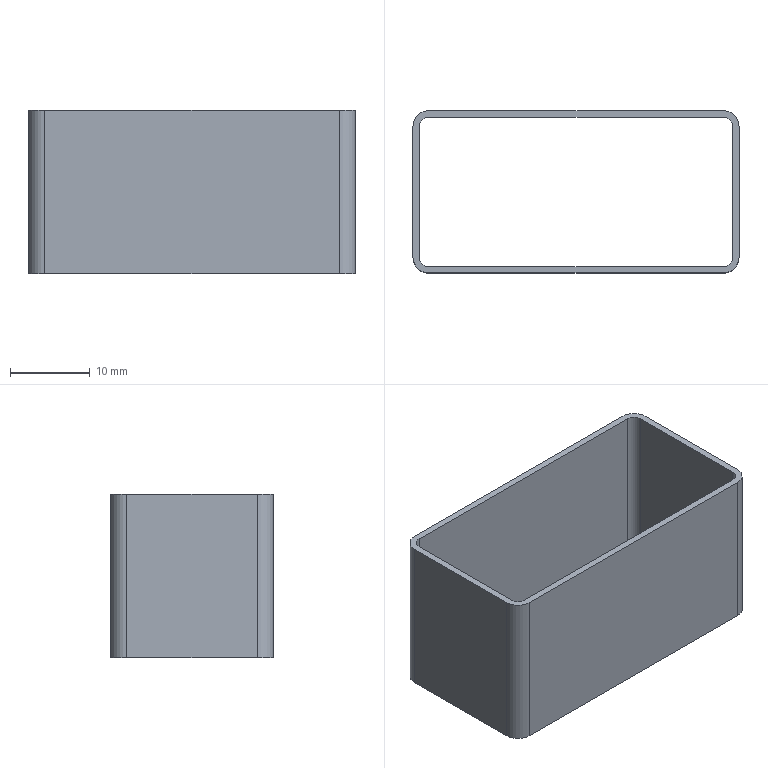Part | STEP file | Zapas-OpenRC Truggy HSPr v2. v55-3 | 1 solid | 18 faces | box 41 x 20.4 x 20.5 mm | volume 1916 mm3 | plane 10 | cylinder 8 | commonest cylinder face diameters 2.4 x4 4 x4
STEP:
#1=CARTESIAN_POINT('',(0.,0.,0.));
#2=DIRECTION('',(0.,0.,1.));
#3=DIRECTION('',(1.,0.,0.));
#4=AXIS2_PLACEMENT_3D('',#1,#2,#3);
#5=CARTESIAN_POINT('',(-21.509,42.508,-107.898));
#6=VERTEX_POINT('',#5);
#7=CARTESIAN_POINT('',(-21.509,42.508,-128.398));
#8=VERTEX_POINT('',#7);
#9=CARTESIAN_POINT('',(-21.509,42.508,-107.898));
#10=DIRECTION('',(0.,0.,-1.));
#11=VECTOR('',#10,1.);
#12=LINE('',#9,#11);
#13=CARTESIAN_POINT('',(-3.009,42.508,-118.148));
#14=DIRECTION('',(0.00000009,-1.,0.));
#15=DIRECTION('',(1.,0.00000009,0.));
#16=AXIS2_PLACEMENT_3D('',#13,#14,#15);
#17=PLANE('',#16);
#18=CARTESIAN_POINT('',(-18.5,10.25));
#19=DIRECTION('',(0.,-1.));
#20=VECTOR('',#19,1.);
#21=LINE('',#18,#20);
#22=(GEOMETRIC_REPRESENTATION_CONTEXT(2)PARAMETRIC_REPRESENTATION_CONTEXT()REPRESENTATION_CONTEXT('',''));
#23=DEFINITIONAL_REPRESENTATION('',(#21),#22);
#24=PCURVE('',#17,#23);
#25=CARTESIAN_POINT('',(-21.509,40.508,-107.898));
#26=DIRECTION('',(0.,0.,-1.));
#27=DIRECTION('',(1.,-0.00000091,0.));
#28=AXIS2_PLACEMENT_3D('',#25,#26,#27);
#29=CYLINDRICAL_SURFACE('',#28,2.);
#30=CARTESIAN_POINT('',(4.712,0.));
#31=DIRECTION('',(0.,1.));
#32=VECTOR('',#31,1.);
#33=LINE('',#30,#32);
#34=(GEOMETRIC_REPRESENTATION_CONTEXT(2)PARAMETRIC_REPRESENTATION_CONTEXT()REPRESENTATION_CONTEXT('',''));
#35=DEFINITIONAL_REPRESENTATION('',(#33),#34);
#36=PCURVE('',#29,#35);
#37=SURFACE_CURVE('',#12,(#24,#36),.PCURVE_S1.);
#38=EDGE_CURVE('',#6,#8,#37,.T.);
#39=ORIENTED_EDGE('',*,*,#38,.F.);
#40=CARTESIAN_POINT('',(15.491,42.508,-107.898));
#41=VERTEX_POINT('',#40);
#42=CARTESIAN_POINT('',(15.491,42.508,-107.898));
#43=DIRECTION('',(-1.,-0.00000009,0.));
#44=VECTOR('',#43,1.);
#45=LINE('',#42,#44);
#46=CARTESIAN_POINT('',(18.5,10.25));
#47=DIRECTION('',(-1.,0.));
#48=VECTOR('',#47,1.);
#49=LINE('',#46,#48);
#50=(GEOMETRIC_REPRESENTATION_CONTEXT(2)PARAMETRIC_REPRESENTATION_CONTEXT()REPRESENTATION_CONTEXT('',''));
#51=DEFINITIONAL_REPRESENTATION('',(#49),#50);
#52=PCURVE('',#17,#51);
#53=CARTESIAN_POINT('',(-3.009,32.308,-107.898));
#54=DIRECTION('',(0.,0.,1.));
#55=DIRECTION('',(-1.,0.00000091,0.));
#56=AXIS2_PLACEMENT_3D('',#53,#54,#55);
#57=PLANE('',#56);
#58=CARTESIAN_POINT('',(-18.5,-10.2));
#59=DIRECTION('',(1.,0.000001));
#60=VECTOR('',#59,1.);
#61=LINE('',#58,#60);
#62=(GEOMETRIC_REPRESENTATION_CONTEXT(2)PARAMETRIC_REPRESENTATION_CONTEXT()REPRESENTATION_CONTEXT('',''));
#63=DEFINITIONAL_REPRESENTATION('',(#61),#62);
#64=PCURVE('',#57,#63);
#65=SURFACE_CURVE('',#45,(#52,#64),.PCURVE_S1.);
#66=EDGE_CURVE('',#41,#6,#65,.T.);
#67=ORIENTED_EDGE('',*,*,#66,.F.);
#68=CARTESIAN_POINT('',(15.491,42.508,-128.398));
#69=VERTEX_POINT('',#68);
#70=CARTESIAN_POINT('',(15.491,42.508,-128.398));
#71=DIRECTION('',(0.,0.,1.));
#72=VECTOR('',#71,1.);
#73=LINE('',#70,#72);
#74=CARTESIAN_POINT('',(18.5,-10.25));
#75=DIRECTION('',(0.,1.));
#76=VECTOR('',#75,1.);
#77=LINE('',#74,#76);
#78=(GEOMETRIC_REPRESENTATION_CONTEXT(2)PARAMETRIC_REPRESENTATION_CONTEXT()REPRESENTATION_CONTEXT('',''));
#79=DEFINITIONAL_REPRESENTATION('',(#77),#78);
#80=PCURVE('',#17,#79);
#81=CARTESIAN_POINT('',(15.491,40.508,-107.898));
#82=DIRECTION('',(0.,0.,-1.));
#83=DIRECTION('',(1.,-0.00000091,0.));
#84=AXIS2_PLACEMENT_3D('',#81,#82,#83);
#85=CYLINDRICAL_SURFACE('',#84,2.);
#86=CARTESIAN_POINT('',(4.712,20.5));
#87=DIRECTION('',(0.,-1.));
#88=VECTOR('',#87,1.);
#89=LINE('',#86,#88);
#90=(GEOMETRIC_REPRESENTATION_CONTEXT(2)PARAMETRIC_REPRESENTATION_CONTEXT()REPRESENTATION_CONTEXT('',''));
#91=DEFINITIONAL_REPRESENTATION('',(#89),#90);
#92=PCURVE('',#85,#91);
#93=SURFACE_CURVE('',#73,(#80,#92),.PCURVE_S1.);
#94=EDGE_CURVE('',#69,#41,#93,.T.);
#95=ORIENTED_EDGE('',*,*,#94,.F.);
#96=CARTESIAN_POINT('',(-21.509,42.508,-128.398));
#97=DIRECTION('',(1.,0.00000009,0.));
#98=VECTOR('',#97,1.);
#99=LINE('',#96,#98);
#100=CARTESIAN_POINT('',(-18.5,-10.25));
#101=DIRECTION('',(1.,0.));
#102=VECTOR('',#101,1.);
#103=LINE('',#100,#102);
#104=(GEOMETRIC_REPRESENTATION_CONTEXT(2)PARAMETRIC_REPRESENTATION_CONTEXT()REPRESENTATION_CONTEXT('',''));
#105=DEFINITIONAL_REPRESENTATION('',(#103),#104);
#106=PCURVE('',#17,#105);
#107=CARTESIAN_POINT('',(-3.009,32.308,-128.398));
#108=DIRECTION('',(0.,0.,1.));
#109=DIRECTION('',(-1.,0.00000091,0.));
#110=AXIS2_PLACEMENT_3D('',#107,#108,#109);
#111=PLANE('',#110);
#112=CARTESIAN_POINT('',(18.5,-10.2));
#113=DIRECTION('',(-1.,-0.000001));
#114=VECTOR('',#113,1.);
#115=LINE('',#112,#114);
#116=(GEOMETRIC_REPRESENTATION_CONTEXT(2)PARAMETRIC_REPRESENTATION_CONTEXT()REPRESENTATION_CONTEXT('',''));
#117=DEFINITIONAL_REPRESENTATION('',(#115),#116);
#118=PCURVE('',#111,#117);
#119=SURFACE_CURVE('',#99,(#106,#118),.PCURVE_S1.);
#120=EDGE_CURVE('',#8,#69,#119,.T.);
#121=ORIENTED_EDGE('',*,*,#120,.F.);
#122=EDGE_LOOP('',(#39,#67,#95,#121));
#123=FACE_BOUND('',#122,.T.);
#124=ADVANCED_FACE('',(#123),#17,.F.);
#125=CARTESIAN_POINT('',(-22.709,40.508,-128.398));
#126=VERTEX_POINT('',#125);
#127=CARTESIAN_POINT('',(-21.509,41.708,-128.398));
#128=VERTEX_POINT('',#127);
#129=CARTESIAN_POINT('',(-21.509,40.508,-128.398));
#130=DIRECTION('',(0.,0.,-1.));
#131=DIRECTION('',(-1.,0.00000091,0.));
#132=AXIS2_PLACEMENT_3D('',#129,#130,#131);
#133=CIRCLE('',#132,1.2);
#134=CARTESIAN_POINT('',(19.7,-8.2));
#135=CARTESIAN_POINT('',(19.7,-10.278));
#136=CARTESIAN_POINT('',(17.9,-9.239));
#137=CARTESIAN_POINT('',(16.1,-8.2));
#138=CARTESIAN_POINT('',(17.9,-7.161));
#139=CARTESIAN_POINT('',(19.7,-6.122));
#140=CARTESIAN_POINT('',(19.7,-8.2));
#141=(BOUNDED_CURVE()B_SPLINE_CURVE(2,(#134,#135,#136,#137,#138,#139,#140),.UNSPECIFIED.,.T.,.F.)B_SPLINE_CURVE_WITH_KNOTS((1,2,2,2,2,1),(-2.094,0.,2.094,4.189,6.283,8.378),.UNSPECIFIED.)CURVE()GEOMETRIC_REPRESENTATION_ITEM()RATIONAL_B_SPLINE_CURVE((1.,0.5,1.,0.5,1.,0.5,1.))REPRESENTATION_ITEM(''));
#142=(GEOMETRIC_REPRESENTATION_CONTEXT(2)PARAMETRIC_REPRESENTATION_CONTEXT()REPRESENTATION_CONTEXT('',''));
#143=DEFINITIONAL_REPRESENTATION('',(#141),#142);
#144=PCURVE('',#111,#143);
#145=CARTESIAN_POINT('',(-21.509,40.508,-128.398));
#146=DIRECTION('',(0.,0.,1.));
#147=DIRECTION('',(-1.,0.00000091,0.));
#148=AXIS2_PLACEMENT_3D('',#145,#146,#147);
#149=CYLINDRICAL_SURFACE('',#148,1.2);
#150=CARTESIAN_POINT('',(12.566,0.));
#151=DIRECTION('',(-1.,0.));
#152=VECTOR('',#151,1.);
#153=LINE('',#150,#152);
#154=(GEOMETRIC_REPRESENTATION_CONTEXT(2)PARAMETRIC_REPRESENTATION_CONTEXT()REPRESENTATION_CONTEXT('',''));
#155=DEFINITIONAL_REPRESENTATION('',(#153),#154);
#156=PCURVE('',#149,#155);
#157=SURFACE_CURVE('',#133,(#144,#156),.PCURVE_S1.);
#158=EDGE_CURVE('',#126,#128,#157,.T.);
#159=ORIENTED_EDGE('',*,*,#158,.F.);
#160=CARTESIAN_POINT('',(-22.709,24.108,-128.398));
#161=VERTEX_POINT('',#160);
#162=CARTESIAN_POINT('',(-22.709,24.108,-128.398));
#163=DIRECTION('',(-0.00000009,1.,0.));
#164=VECTOR('',#163,1.);
#165=LINE('',#162,#164);
#166=CARTESIAN_POINT('',(19.7,8.2));
#167=DIRECTION('',(0.000001,-1.));
#168=VECTOR('',#167,1.);
#169=LINE('',#166,#168);
#170=(GEOMETRIC_REPRESENTATION_CONTEXT(2)PARAMETRIC_REPRESENTATION_CONTEXT()REPRESENTATION_CONTEXT('',''));
#171=DEFINITIONAL_REPRESENTATION('',(#169),#170);
#172=PCURVE('',#111,#171);
#173=CARTESIAN_POINT('',(-22.709,32.308,-118.148));
#174=DIRECTION('',(-1.,-0.00000009,0.));
#175=DIRECTION('',(0.00000009,-1.,0.));
#176=AXIS2_PLACEMENT_3D('',#173,#174,#175);
#177=PLANE('',#176);
#178=CARTESIAN_POINT('',(8.2,-10.25));
#179=DIRECTION('',(-1.,0.));
#180=VECTOR('',#179,1.);
#181=LINE('',#178,#180);
#182=(GEOMETRIC_REPRESENTATION_CONTEXT(2)PARAMETRIC_REPRESENTATION_CONTEXT()REPRESENTATION_CONTEXT('',''));
#183=DEFINITIONAL_REPRESENTATION('',(#181),#182);
#184=PCURVE('',#177,#183);
#185=SURFACE_CURVE('',#165,(#172,#184),.PCURVE_S1.);
#186=EDGE_CURVE('',#161,#126,#185,.T.);
#187=ORIENTED_EDGE('',*,*,#186,.F.);
#188=CARTESIAN_POINT('',(-21.509,22.908,-128.398));
#189=VERTEX_POINT('',#188);
#190=CARTESIAN_POINT('',(-21.509,24.108,-128.398));
#191=DIRECTION('',(0.,0.,-1.));
#192=DIRECTION('',(-1.,0.00000091,0.));
#193=AXIS2_PLACEMENT_3D('',#190,#191,#192);
#194=CIRCLE('',#193,1.2);
#195=CARTESIAN_POINT('',(19.7,8.2));
#196=CARTESIAN_POINT('',(19.7,6.122));
#197=CARTESIAN_POINT('',(17.9,7.161));
#198=CARTESIAN_POINT('',(16.1,8.2));
#199=CARTESIAN_POINT('',(17.9,9.239));
#200=CARTESIAN_POINT('',(19.7,10.278));
#201=CARTESIAN_POINT('',(19.7,8.2));
#202=(BOUNDED_CURVE()B_SPLINE_CURVE(2,(#195,#196,#197,#198,#199,#200,#201),.UNSPECIFIED.,.T.,.F.)B_SPLINE_CURVE_WITH_KNOTS((1,2,2,2,2,1),(-2.094,0.,2.094,4.189,6.283,8.378),.UNSPECIFIED.)CURVE()GEOMETRIC_REPRESENTATION_ITEM()RATIONAL_B_SPLINE_CURVE((1.,0.5,1.,0.5,1.,0.5,1.))REPRESENTATION_ITEM(''));
#203=(GEOMETRIC_REPRESENTATION_CONTEXT(2)PARAMETRIC_REPRESENTATION_CONTEXT()REPRESENTATION_CONTEXT('',''));
#204=DEFINITIONAL_REPRESENTATION('',(#202),#203);
#205=PCURVE('',#111,#204);
#206=CARTESIAN_POINT('',(-21.509,24.108,-128.398));
#207=DIRECTION('',(0.,0.,1.));
#208=DIRECTION('',(-1.,0.00000091,0.));
#209=AXIS2_PLACEMENT_3D('',#206,#207,#208);
#210=CYLINDRICAL_SURFACE('',#209,1.2);
#211=CARTESIAN_POINT('',(6.283,0.));
#212=DIRECTION('',(-1.,0.));
#213=VECTOR('',#212,1.);
#214=LINE('',#211,#213);
#215=(GEOMETRIC_REPRESENTATION_CONTEXT(2)PARAMETRIC_REPRESENTATION_CONTEXT()REPRESENTATION_CONTEXT('',''));
#216=DEFINITIONAL_REPRESENTATION('',(#214),#215);
#217=PCURVE('',#210,#216);
#218=SURFACE_CURVE('',#194,(#205,#217),.PCURVE_S1.);
#219=EDGE_CURVE('',#189,#161,#218,.T.);
#220=ORIENTED_EDGE('',*,*,#219,.F.);
#221=CARTESIAN_POINT('',(15.491,22.908,-128.398));
#222=VERTEX_POINT('',#221);
#223=CARTESIAN_POINT('',(15.491,22.908,-128.398));
#224=DIRECTION('',(-1.,-0.00000009,0.));
#225=VECTOR('',#224,1.);
#226=LINE('',#223,#225);
#227=CARTESIAN_POINT('',(-18.5,9.4));
#228=DIRECTION('',(1.,0.000001));
#229=VECTOR('',#228,1.);
#230=LINE('',#227,#229);
#231=(GEOMETRIC_REPRESENTATION_CONTEXT(2)PARAMETRIC_REPRESENTATION_CONTEXT()REPRESENTATION_CONTEXT('',''));
#232=DEFINITIONAL_REPRESENTATION('',(#230),#231);
#233=PCURVE('',#111,#232);
#234=CARTESIAN_POINT('',(-3.009,22.908,-118.148));
#235=DIRECTION('',(0.00000009,-1.,0.));
#236=DIRECTION('',(1.,0.00000009,0.));
#237=AXIS2_PLACEMENT_3D('',#234,#235,#236);
#238=PLANE('',#237);
#239=CARTESIAN_POINT('',(18.5,-10.25));
#240=DIRECTION('',(-1.,0.));
#241=VECTOR('',#240,1.);
#242=LINE('',#239,#241);
#243=(GEOMETRIC_REPRESENTATION_CONTEXT(2)PARAMETRIC_REPRESENTATION_CONTEXT()REPRESENTATION_CONTEXT('',''));
#244=DEFINITIONAL_REPRESENTATION('',(#242),#243);
#245=PCURVE('',#238,#244);
#246=SURFACE_CURVE('',#226,(#233,#245),.PCURVE_S1.);
#247=EDGE_CURVE('',#222,#189,#246,.T.);
#248=ORIENTED_EDGE('',*,*,#247,.F.);
#249=CARTESIAN_POINT('',(16.691,24.108,-128.398));
#250=VERTEX_POINT('',#249);
#251=CARTESIAN_POINT('',(15.491,24.108,-128.398));
#252=DIRECTION('',(0.,0.,-1.));
#253=DIRECTION('',(-1.,0.00000091,0.));
#254=AXIS2_PLACEMENT_3D('',#251,#252,#253);
#255=CIRCLE('',#254,1.2);
#256=CARTESIAN_POINT('',(-17.3,8.2));
#257=CARTESIAN_POINT('',(-17.3,6.122));
#258=CARTESIAN_POINT('',(-19.1,7.161));
#259=CARTESIAN_POINT('',(-20.9,8.2));
#260=CARTESIAN_POINT('',(-19.1,9.239));
#261=CARTESIAN_POINT('',(-17.3,10.278));
#262=CARTESIAN_POINT('',(-17.3,8.2));
#263=(BOUNDED_CURVE()B_SPLINE_CURVE(2,(#256,#257,#258,#259,#260,#261,#262),.UNSPECIFIED.,.T.,.F.)B_SPLINE_CURVE_WITH_KNOTS((1,2,2,2,2,1),(-2.094,0.,2.094,4.189,6.283,8.378),.UNSPECIFIED.)CURVE()GEOMETRIC_REPRESENTATION_ITEM()RATIONAL_B_SPLINE_CURVE((1.,0.5,1.,0.5,1.,0.5,1.))REPRESENTATION_ITEM(''));
#264=(GEOMETRIC_REPRESENTATION_CONTEXT(2)PARAMETRIC_REPRESENTATION_CONTEXT()REPRESENTATION_CONTEXT('',''));
#265=DEFINITIONAL_REPRESENTATION('',(#263),#264);
#266=PCURVE('',#111,#265);
#267=CARTESIAN_POINT('',(15.491,24.108,-128.398));
#268=DIRECTION('',(0.,0.,1.));
#269=DIRECTION('',(-1.,0.00000091,0.));
#270=AXIS2_PLACEMENT_3D('',#267,#268,#269);
#271=CYLINDRICAL_SURFACE('',#270,1.2);
#272=CARTESIAN_POINT('',(6.283,0.));
#273=DIRECTION('',(-1.,0.));
#274=VECTOR('',#273,1.);
#275=LINE('',#272,#274);
#276=(GEOMETRIC_REPRESENTATION_CONTEXT(2)PARAMETRIC_REPRESENTATION_CONTEXT()REPRESENTATION_CONTEXT('',''));
#277=DEFINITIONAL_REPRESENTATION('',(#275),#276);
#278=PCURVE('',#271,#277);
#279=SURFACE_CURVE('',#255,(#266,#278),.PCURVE_S1.);
#280=EDGE_CURVE('',#250,#222,#279,.T.);
#281=ORIENTED_EDGE('',*,*,#280,.F.);
#282=CARTESIAN_POINT('',(16.691,40.508,-128.398));
#283=VERTEX_POINT('',#282);
#284=CARTESIAN_POINT('',(16.691,40.508,-128.398));
#285=DIRECTION('',(0.00000009,-1.,0.));
#286=VECTOR('',#285,1.);
#287=LINE('',#284,#286);
#288=CARTESIAN_POINT('',(-19.7,-8.2));
#289=DIRECTION('',(-0.000001,1.));
#290=VECTOR('',#289,1.);
#291=LINE('',#288,#290);
#292=(GEOMETRIC_REPRESENTATION_CONTEXT(2)PARAMETRIC_REPRESENTATION_CONTEXT()REPRESENTATION_CONTEXT('',''));
#293=DEFINITIONAL_REPRESENTATION('',(#291),#292);
#294=PCURVE('',#111,#293);
#295=CARTESIAN_POINT('',(16.691,32.308,-118.148));
#296=DIRECTION('',(1.,0.00000009,0.));
#297=DIRECTION('',(-0.00000009,1.,0.));
#298=AXIS2_PLACEMENT_3D('',#295,#296,#297);
#299=PLANE('',#298);
#300=CARTESIAN_POINT('',(8.2,-10.25));
#301=DIRECTION('',(-1.,0.));
#302=VECTOR('',#301,1.);
#303=LINE('',#300,#302);
#304=(GEOMETRIC_REPRESENTATION_CONTEXT(2)PARAMETRIC_REPRESENTATION_CONTEXT()REPRESENTATION_CONTEXT('',''));
#305=DEFINITIONAL_REPRESENTATION('',(#303),#304);
#306=PCURVE('',#299,#305);
#307=SURFACE_CURVE('',#287,(#294,#306),.PCURVE_S1.);
#308=EDGE_CURVE('',#283,#250,#307,.T.);
#309=ORIENTED_EDGE('',*,*,#308,.F.);
#310=CARTESIAN_POINT('',(15.491,41.708,-128.398));
#311=VERTEX_POINT('',#310);
#312=CARTESIAN_POINT('',(15.491,40.508,-128.398));
#313=DIRECTION('',(0.,0.,-1.));
#314=DIRECTION('',(-1.,0.00000091,0.));
#315=AXIS2_PLACEMENT_3D('',#312,#313,#314);
#316=CIRCLE('',#315,1.2);
#317=CARTESIAN_POINT('',(-17.3,-8.2));
#318=CARTESIAN_POINT('',(-17.3,-10.278));
#319=CARTESIAN_POINT('',(-19.1,-9.239));
#320=CARTESIAN_POINT('',(-20.9,-8.2));
#321=CARTESIAN_POINT('',(-19.1,-7.161));
#322=CARTESIAN_POINT('',(-17.3,-6.122));
#323=CARTESIAN_POINT('',(-17.3,-8.2));
#324=(BOUNDED_CURVE()B_SPLINE_CURVE(2,(#317,#318,#319,#320,#321,#322,#323),.UNSPECIFIED.,.T.,.F.)B_SPLINE_CURVE_WITH_KNOTS((1,2,2,2,2,1),(-2.094,0.,2.094,4.189,6.283,8.378),.UNSPECIFIED.)CURVE()GEOMETRIC_REPRESENTATION_ITEM()RATIONAL_B_SPLINE_CURVE((1.,0.5,1.,0.5,1.,0.5,1.))REPRESENTATION_ITEM(''));
#325=(GEOMETRIC_REPRESENTATION_CONTEXT(2)PARAMETRIC_REPRESENTATION_CONTEXT()REPRESENTATION_CONTEXT('',''));
#326=DEFINITIONAL_REPRESENTATION('',(#324),#325);
#327=PCURVE('',#111,#326);
#328=CARTESIAN_POINT('',(15.491,40.508,-128.398));
#329=DIRECTION('',(0.,0.,1.));
#330=DIRECTION('',(-1.,0.00000091,0.));
#331=AXIS2_PLACEMENT_3D('',#328,#329,#330);
#332=CYLINDRICAL_SURFACE('',#331,1.2);
#333=CARTESIAN_POINT('',(6.283,0.));
#334=DIRECTION('',(-1.,0.));
#335=VECTOR('',#334,1.);
#336=LINE('',#333,#335);
#337=(GEOMETRIC_REPRESENTATION_CONTEXT(2)PARAMETRIC_REPRESENTATION_CONTEXT()REPRESENTATION_CONTEXT('',''));
#338=DEFINITIONAL_REPRESENTATION('',(#336),#337);
#339=PCURVE('',#332,#338);
#340=SURFACE_CURVE('',#316,(#327,#339),.PCURVE_S1.);
#341=EDGE_CURVE('',#311,#283,#340,.T.);
#342=ORIENTED_EDGE('',*,*,#341,.F.);
#343=CARTESIAN_POINT('',(-21.509,41.708,-128.398));
#344=DIRECTION('',(1.,0.00000009,0.));
#345=VECTOR('',#344,1.);
#346=LINE('',#343,#345);
#347=CARTESIAN_POINT('',(18.5,-9.4));
#348=DIRECTION('',(-1.,-0.000001));
#349=VECTOR('',#348,1.);
#350=LINE('',#347,#349);
#351=(GEOMETRIC_REPRESENTATION_CONTEXT(2)PARAMETRIC_REPRESENTATION_CONTEXT()REPRESENTATION_CONTEXT('',''));
#352=DEFINITIONAL_REPRESENTATION('',(#350),#351);
#353=PCURVE('',#111,#352);
#354=CARTESIAN_POINT('',(-3.009,41.708,-118.148));
#355=DIRECTION('',(-0.00000009,1.,0.));
#356=DIRECTION('',(-1.,-0.00000009,0.));
#357=AXIS2_PLACEMENT_3D('',#354,#355,#356);
#358=PLANE('',#357);
#359=CARTESIAN_POINT('',(18.5,-10.25));
#360=DIRECTION('',(-1.,0.));
#361=VECTOR('',#360,1.);
#362=LINE('',#359,#361);
#363=(GEOMETRIC_REPRESENTATION_CONTEXT(2)PARAMETRIC_REPRESENTATION_CONTEXT()REPRESENTATION_CONTEXT('',''));
#364=DEFINITIONAL_REPRESENTATION('',(#362),#363);
#365=PCURVE('',#358,#364);
#366=SURFACE_CURVE('',#346,(#353,#365),.PCURVE_S1.);
#367=EDGE_CURVE('',#128,#311,#366,.T.);
#368=ORIENTED_EDGE('',*,*,#367,.F.);
#369=EDGE_LOOP('',(#159,#187,#220,#248,#281,#309,#342,#368));
#370=FACE_BOUND('',#369,.T.);
#371=CARTESIAN_POINT('',(-23.509,24.108,-128.398));
#372=VERTEX_POINT('',#371);
#373=CARTESIAN_POINT('',(-21.509,22.108,-128.398));
#374=VERTEX_POINT('',#373);
#375=CARTESIAN_POINT('',(-21.509,24.108,-128.398));
#376=DIRECTION('',(0.,0.,1.));
#377=DIRECTION('',(1.,-0.00000091,0.));
#378=AXIS2_PLACEMENT_3D('',#375,#376,#377);
#379=CIRCLE('',#378,2.);
#380=CARTESIAN_POINT('',(18.5,8.2));
#381=DIRECTION('',(-1.,0.));
#382=AXIS2_PLACEMENT_2D('',#380,#381);
#383=CIRCLE('',#382,2.);
#384=(GEOMETRIC_REPRESENTATION_CONTEXT(2)PARAMETRIC_REPRESENTATION_CONTEXT()REPRESENTATION_CONTEXT('',''));
#385=DEFINITIONAL_REPRESENTATION('',(#383),#384);
#386=PCURVE('',#111,#385);
#387=CARTESIAN_POINT('',(-21.509,24.108,-107.898));
#388=DIRECTION('',(0.,0.,-1.));
#389=DIRECTION('',(1.,-0.00000091,0.));
#390=AXIS2_PLACEMENT_3D('',#387,#388,#389);
#391=CYLINDRICAL_SURFACE('',#390,2.);
#392=CARTESIAN_POINT('',(6.283,20.5));
#393=DIRECTION('',(-1.,0.));
#394=VECTOR('',#393,1.);
#395=LINE('',#392,#394);
#396=(GEOMETRIC_REPRESENTATION_CONTEXT(2)PARAMETRIC_REPRESENTATION_CONTEXT()REPRESENTATION_CONTEXT('',''));
#397=DEFINITIONAL_REPRESENTATION('',(#395),#396);
#398=PCURVE('',#391,#397);
#399=SURFACE_CURVE('',#379,(#386,#398),.PCURVE_S1.);
#400=EDGE_CURVE('',#372,#374,#399,.T.);
#401=ORIENTED_EDGE('',*,*,#400,.F.);
#402=CARTESIAN_POINT('',(-23.509,40.508,-128.398));
#403=VERTEX_POINT('',#402);
#404=CARTESIAN_POINT('',(-23.509,40.508,-128.398));
#405=DIRECTION('',(0.00000009,-1.,0.));
#406=VECTOR('',#405,1.);
#407=LINE('',#404,#406);
#408=CARTESIAN_POINT('',(20.5,-8.2));
#409=DIRECTION('',(-0.000001,1.));
#410=VECTOR('',#409,1.);
#411=LINE('',#408,#410);
#412=(GEOMETRIC_REPRESENTATION_CONTEXT(2)PARAMETRIC_REPRESENTATION_CONTEXT()REPRESENTATION_CONTEXT('',''));
#413=DEFINITIONAL_REPRESENTATION('',(#411),#412);
#414=PCURVE('',#111,#413);
#415=CARTESIAN_POINT('',(-23.509,32.308,-118.148));
#416=DIRECTION('',(1.,0.00000009,0.));
#417=DIRECTION('',(-0.00000009,1.,0.));
#418=AXIS2_PLACEMENT_3D('',#415,#416,#417);
#419=PLANE('',#418);
#420=CARTESIAN_POINT('',(8.2,-10.25));
#421=DIRECTION('',(-1.,0.));
#422=VECTOR('',#421,1.);
#423=LINE('',#420,#422);
#424=(GEOMETRIC_REPRESENTATION_CONTEXT(2)PARAMETRIC_REPRESENTATION_CONTEXT()REPRESENTATION_CONTEXT('',''));
#425=DEFINITIONAL_REPRESENTATION('',(#423),#424);
#426=PCURVE('',#419,#425);
#427=SURFACE_CURVE('',#407,(#414,#426),.PCURVE_S1.);
#428=EDGE_CURVE('',#403,#372,#427,.T.);
#429=ORIENTED_EDGE('',*,*,#428,.F.);
#430=CARTESIAN_POINT('',(-21.509,40.508,-128.398));
#431=DIRECTION('',(0.,0.,1.));
#432=DIRECTION('',(1.,-0.00000091,0.));
#433=AXIS2_PLACEMENT_3D('',#430,#431,#432);
#434=CIRCLE('',#433,2.);
#435=CARTESIAN_POINT('',(18.5,-8.2));
#436=DIRECTION('',(-1.,0.));
#437=AXIS2_PLACEMENT_2D('',#435,#436);
#438=CIRCLE('',#437,2.);
#439=(GEOMETRIC_REPRESENTATION_CONTEXT(2)PARAMETRIC_REPRESENTATION_CONTEXT()REPRESENTATION_CONTEXT('',''));
#440=DEFINITIONAL_REPRESENTATION('',(#438),#439);
#441=PCURVE('',#111,#440);
#442=CARTESIAN_POINT('',(6.283,20.5));
#443=DIRECTION('',(-1.,0.));
#444=VECTOR('',#443,1.);
#445=LINE('',#442,#444);
#446=(GEOMETRIC_REPRESENTATION_CONTEXT(2)PARAMETRIC_REPRESENTATION_CONTEXT()REPRESENTATION_CONTEXT('',''));
#447=DEFINITIONAL_REPRESENTATION('',(#445),#446);
#448=PCURVE('',#29,#447);
#449=SURFACE_CURVE('',#434,(#441,#448),.PCURVE_S1.);
#450=EDGE_CURVE('',#8,#403,#449,.T.);
#451=ORIENTED_EDGE('',*,*,#450,.F.);
#452=ORIENTED_EDGE('',*,*,#120,.T.);
#453=CARTESIAN_POINT('',(17.491,40.508,-128.398));
#454=VERTEX_POINT('',#453);
#455=CARTESIAN_POINT('',(15.491,40.508,-128.398));
#456=DIRECTION('',(0.,0.,1.));
#457=DIRECTION('',(1.,-0.00000091,0.));
#458=AXIS2_PLACEMENT_3D('',#455,#456,#457);
#459=CIRCLE('',#458,2.);
#460=CARTESIAN_POINT('',(-18.5,-8.2));
#461=DIRECTION('',(-1.,0.));
#462=AXIS2_PLACEMENT_2D('',#460,#461);
#463=CIRCLE('',#462,2.);
#464=(GEOMETRIC_REPRESENTATION_CONTEXT(2)PARAMETRIC_REPRESENTATION_CONTEXT()REPRESENTATION_CONTEXT('',''));
#465=DEFINITIONAL_REPRESENTATION('',(#463),#464);
#466=PCURVE('',#111,#465);
#467=CARTESIAN_POINT('',(6.283,20.5));
#468=DIRECTION('',(-1.,0.));
#469=VECTOR('',#468,1.);
#470=LINE('',#467,#469);
#471=(GEOMETRIC_REPRESENTATION_CONTEXT(2)PARAMETRIC_REPRESENTATION_CONTEXT()REPRESENTATION_CONTEXT('',''));
#472=DEFINITIONAL_REPRESENTATION('',(#470),#471);
#473=PCURVE('',#85,#472);
#474=SURFACE_CURVE('',#459,(#466,#473),.PCURVE_S1.);
#475=EDGE_CURVE('',#454,#69,#474,.T.);
#476=ORIENTED_EDGE('',*,*,#475,.F.);
#477=CARTESIAN_POINT('',(17.491,24.108,-128.398));
#478=VERTEX_POINT('',#477);
#479=CARTESIAN_POINT('',(17.491,24.108,-128.398));
#480=DIRECTION('',(-0.00000009,1.,0.));
#481=VECTOR('',#480,1.);
#482=LINE('',#479,#481);
#483=CARTESIAN_POINT('',(-20.5,8.2));
#484=DIRECTION('',(0.000001,-1.));
#485=VECTOR('',#484,1.);
#486=LINE('',#483,#485);
#487=(GEOMETRIC_REPRESENTATION_CONTEXT(2)PARAMETRIC_REPRESENTATION_CONTEXT()REPRESENTATION_CONTEXT('',''));
#488=DEFINITIONAL_REPRESENTATION('',(#486),#487);
#489=PCURVE('',#111,#488);
#490=CARTESIAN_POINT('',(17.491,32.308,-118.148));
#491=DIRECTION('',(-1.,-0.00000009,0.));
#492=DIRECTION('',(0.00000009,-1.,0.));
#493=AXIS2_PLACEMENT_3D('',#490,#491,#492);
#494=PLANE('',#493);
#495=CARTESIAN_POINT('',(8.2,-10.25));
#496=DIRECTION('',(-1.,0.));
#497=VECTOR('',#496,1.);
#498=LINE('',#495,#497);
#499=(GEOMETRIC_REPRESENTATION_CONTEXT(2)PARAMETRIC_REPRESENTATION_CONTEXT()REPRESENTATION_CONTEXT('',''));
#500=DEFINITIONAL_REPRESENTATION('',(#498),#499);
#501=PCURVE('',#494,#500);
#502=SURFACE_CURVE('',#482,(#489,#501),.PCURVE_S1.);
#503=EDGE_CURVE('',#478,#454,#502,.T.);
#504=ORIENTED_EDGE('',*,*,#503,.F.);
#505=CARTESIAN_POINT('',(15.491,22.108,-128.398));
#506=VERTEX_POINT('',#505);
#507=CARTESIAN_POINT('',(15.491,24.108,-128.398));
#508=DIRECTION('',(0.,0.,1.));
#509=DIRECTION('',(1.,-0.00000091,0.));
#510=AXIS2_PLACEMENT_3D('',#507,#508,#509);
#511=CIRCLE('',#510,2.);
#512=CARTESIAN_POINT('',(-18.5,8.2));
#513=DIRECTION('',(-1.,0.));
#514=AXIS2_PLACEMENT_2D('',#512,#513);
#515=CIRCLE('',#514,2.);
#516=(GEOMETRIC_REPRESENTATION_CONTEXT(2)PARAMETRIC_REPRESENTATION_CONTEXT()REPRESENTATION_CONTEXT('',''));
#517=DEFINITIONAL_REPRESENTATION('',(#515),#516);
#518=PCURVE('',#111,#517);
#519=CARTESIAN_POINT('',(15.491,24.108,-107.898));
#520=DIRECTION('',(0.,0.,-1.));
#521=DIRECTION('',(1.,-0.00000091,0.));
#522=AXIS2_PLACEMENT_3D('',#519,#520,#521);
#523=CYLINDRICAL_SURFACE('',#522,2.);
#524=CARTESIAN_POINT('',(6.283,20.5));
#525=DIRECTION('',(-1.,0.));
#526=VECTOR('',#525,1.);
#527=LINE('',#524,#526);
#528=(GEOMETRIC_REPRESENTATION_CONTEXT(2)PARAMETRIC_REPRESENTATION_CONTEXT()REPRESENTATION_CONTEXT('',''));
#529=DEFINITIONAL_REPRESENTATION('',(#527),#528);
#530=PCURVE('',#523,#529);
#531=SURFACE_CURVE('',#511,(#518,#530),.PCURVE_S1.);
#532=EDGE_CURVE('',#506,#478,#531,.T.);
#533=ORIENTED_EDGE('',*,*,#532,.F.);
#534=CARTESIAN_POINT('',(-21.509,22.108,-128.398));
#535=DIRECTION('',(1.,0.00000009,0.));
#536=VECTOR('',#535,1.);
#537=LINE('',#534,#536);
#538=CARTESIAN_POINT('',(18.5,10.2));
#539=DIRECTION('',(-1.,-0.000001));
#540=VECTOR('',#539,1.);
#541=LINE('',#538,#540);
#542=(GEOMETRIC_REPRESENTATION_CONTEXT(2)PARAMETRIC_REPRESENTATION_CONTEXT()REPRESENTATION_CONTEXT('',''));
#543=DEFINITIONAL_REPRESENTATION('',(#541),#542);
#544=PCURVE('',#111,#543);
#545=CARTESIAN_POINT('',(-3.009,22.108,-118.148));
#546=DIRECTION('',(-0.00000009,1.,0.));
#547=DIRECTION('',(-1.,-0.00000009,0.));
#548=AXIS2_PLACEMENT_3D('',#545,#546,#547);
#549=PLANE('',#548);
#550=CARTESIAN_POINT('',(18.5,-10.25));
#551=DIRECTION('',(-1.,0.));
#552=VECTOR('',#551,1.);
#553=LINE('',#550,#552);
#554=(GEOMETRIC_REPRESENTATION_CONTEXT(2)PARAMETRIC_REPRESENTATION_CONTEXT()REPRESENTATION_CONTEXT('',''));
#555=DEFINITIONAL_REPRESENTATION('',(#553),#554);
#556=PCURVE('',#549,#555);
#557=SURFACE_CURVE('',#537,(#544,#556),.PCURVE_S1.);
#558=EDGE_CURVE('',#374,#506,#557,.T.);
#559=ORIENTED_EDGE('',*,*,#558,.F.);
#560=EDGE_LOOP('',(#401,#429,#451,#452,#476,#504,#533,#559));
#561=FACE_BOUND('',#560,.T.);
#562=ADVANCED_FACE('',(#370,#561),#111,.F.);
#563=ORIENTED_EDGE('',*,*,#450,.T.);
#564=CARTESIAN_POINT('',(-23.509,40.508,-107.898));
#565=VERTEX_POINT('',#564);
#566=CARTESIAN_POINT('',(-23.509,40.508,-128.398));
#567=DIRECTION('',(0.,0.,1.));
#568=VECTOR('',#567,1.);
#569=LINE('',#566,#568);
#570=CARTESIAN_POINT('',(3.142,20.5));
#571=DIRECTION('',(0.,-1.));
#572=VECTOR('',#571,1.);
#573=LINE('',#570,#572);
#574=(GEOMETRIC_REPRESENTATION_CONTEXT(2)PARAMETRIC_REPRESENTATION_CONTEXT()REPRESENTATION_CONTEXT('',''));
#575=DEFINITIONAL_REPRESENTATION('',(#573),#574);
#576=PCURVE('',#29,#575);
#577=CARTESIAN_POINT('',(8.2,-10.25));
#578=DIRECTION('',(0.,1.));
#579=VECTOR('',#578,1.);
#580=LINE('',#577,#579);
#581=(GEOMETRIC_REPRESENTATION_CONTEXT(2)PARAMETRIC_REPRESENTATION_CONTEXT()REPRESENTATION_CONTEXT('',''));
#582=DEFINITIONAL_REPRESENTATION('',(#580),#581);
#583=PCURVE('',#419,#582);
#584=SURFACE_CURVE('',#569,(#576,#583),.PCURVE_S1.);
#585=EDGE_CURVE('',#403,#565,#584,.T.);
#586=ORIENTED_EDGE('',*,*,#585,.T.);
#587=CARTESIAN_POINT('',(-21.509,40.508,-107.898));
#588=DIRECTION('',(0.,0.,-1.));
#589=DIRECTION('',(1.,-0.00000091,0.));
#590=AXIS2_PLACEMENT_3D('',#587,#588,#589);
#591=CIRCLE('',#590,2.);
#592=CARTESIAN_POINT('',(0.,0.));
#593=DIRECTION('',(1.,0.));
#594=VECTOR('',#593,1.);
#595=LINE('',#592,#594);
#596=(GEOMETRIC_REPRESENTATION_CONTEXT(2)PARAMETRIC_REPRESENTATION_CONTEXT()REPRESENTATION_CONTEXT('',''));
#597=DEFINITIONAL_REPRESENTATION('',(#595),#596);
#598=PCURVE('',#29,#597);
#599=CARTESIAN_POINT('',(16.5,-8.2));
#600=CARTESIAN_POINT('',(16.5,-4.736));
#601=CARTESIAN_POINT('',(19.5,-6.468));
#602=CARTESIAN_POINT('',(22.5,-8.2));
#603=CARTESIAN_POINT('',(19.5,-9.932));
#604=CARTESIAN_POINT('',(16.5,-11.664));
#605=CARTESIAN_POINT('',(16.5,-8.2));
#606=(BOUNDED_CURVE()B_SPLINE_CURVE(2,(#599,#600,#601,#602,#603,#604,#605),.UNSPECIFIED.,.T.,.F.)B_SPLINE_CURVE_WITH_KNOTS((1,2,2,2,2,1),(-2.094,0.,2.094,4.189,6.283,8.378),.UNSPECIFIED.)CURVE()GEOMETRIC_REPRESENTATION_ITEM()RATIONAL_B_SPLINE_CURVE((1.,0.5,1.,0.5,1.,0.5,1.))REPRESENTATION_ITEM(''));
#607=(GEOMETRIC_REPRESENTATION_CONTEXT(2)PARAMETRIC_REPRESENTATION_CONTEXT()REPRESENTATION_CONTEXT('',''));
#608=DEFINITIONAL_REPRESENTATION('',(#606),#607);
#609=PCURVE('',#57,#608);
#610=SURFACE_CURVE('',#591,(#598,#609),.PCURVE_S1.);
#611=EDGE_CURVE('',#565,#6,#610,.T.);
#612=ORIENTED_EDGE('',*,*,#611,.T.);
#613=ORIENTED_EDGE('',*,*,#38,.T.);
#614=EDGE_LOOP('',(#563,#586,#612,#613));
#615=FACE_BOUND('',#614,.T.);
#616=ADVANCED_FACE('',(#615),#29,.T.);
#617=CARTESIAN_POINT('',(-21.509,22.908,-107.898));
#618=VERTEX_POINT('',#617);
#619=CARTESIAN_POINT('',(-22.709,24.108,-107.898));
#620=VERTEX_POINT('',#619);
#621=CARTESIAN_POINT('',(-21.509,24.108,-107.898));
#622=DIRECTION('',(0.,0.,-1.));
#623=DIRECTION('',(-1.,0.00000091,0.));
#624=AXIS2_PLACEMENT_3D('',#621,#622,#623);
#625=CIRCLE('',#624,1.2);
#626=CARTESIAN_POINT('',(19.7,8.2));
#627=CARTESIAN_POINT('',(19.7,6.122));
#628=CARTESIAN_POINT('',(17.9,7.161));
#629=CARTESIAN_POINT('',(16.1,8.2));
#630=CARTESIAN_POINT('',(17.9,9.239));
#631=CARTESIAN_POINT('',(19.7,10.278));
#632=CARTESIAN_POINT('',(19.7,8.2));
#633=(BOUNDED_CURVE()B_SPLINE_CURVE(2,(#626,#627,#628,#629,#630,#631,#632),.UNSPECIFIED.,.T.,.F.)B_SPLINE_CURVE_WITH_KNOTS((1,2,2,2,2,1),(-2.094,0.,2.094,4.189,6.283,8.378),.UNSPECIFIED.)CURVE()GEOMETRIC_REPRESENTATION_ITEM()RATIONAL_B_SPLINE_CURVE((1.,0.5,1.,0.5,1.,0.5,1.))REPRESENTATION_ITEM(''));
#634=(GEOMETRIC_REPRESENTATION_CONTEXT(2)PARAMETRIC_REPRESENTATION_CONTEXT()REPRESENTATION_CONTEXT('',''));
#635=DEFINITIONAL_REPRESENTATION('',(#633),#634);
#636=PCURVE('',#57,#635);
#637=CARTESIAN_POINT('',(6.283,20.5));
#638=DIRECTION('',(-1.,0.));
#639=VECTOR('',#638,1.);
#640=LINE('',#637,#639);
#641=(GEOMETRIC_REPRESENTATION_CONTEXT(2)PARAMETRIC_REPRESENTATION_CONTEXT()REPRESENTATION_CONTEXT('',''));
#642=DEFINITIONAL_REPRESENTATION('',(#640),#641);
#643=PCURVE('',#210,#642);
#644=SURFACE_CURVE('',#625,(#636,#643),.PCURVE_S1.);
#645=EDGE_CURVE('',#618,#620,#644,.T.);
#646=ORIENTED_EDGE('',*,*,#645,.T.);
#647=CARTESIAN_POINT('',(-22.709,40.508,-107.898));
#648=VERTEX_POINT('',#647);
#649=CARTESIAN_POINT('',(-22.709,24.108,-107.898));
#650=DIRECTION('',(-0.00000009,1.,0.));
#651=VECTOR('',#650,1.);
#652=LINE('',#649,#651);
#653=CARTESIAN_POINT('',(19.7,8.2));
#654=DIRECTION('',(0.000001,-1.));
#655=VECTOR('',#654,1.);
#656=LINE('',#653,#655);
#657=(GEOMETRIC_REPRESENTATION_CONTEXT(2)PARAMETRIC_REPRESENTATION_CONTEXT()REPRESENTATION_CONTEXT('',''));
#658=DEFINITIONAL_REPRESENTATION('',(#656),#657);
#659=PCURVE('',#57,#658);
#660=CARTESIAN_POINT('',(8.2,10.25));
#661=DIRECTION('',(-1.,0.));
#662=VECTOR('',#661,1.);
#663=LINE('',#660,#662);
#664=(GEOMETRIC_REPRESENTATION_CONTEXT(2)PARAMETRIC_REPRESENTATION_CONTEXT()REPRESENTATION_CONTEXT('',''));
#665=DEFINITIONAL_REPRESENTATION('',(#663),#664);
#666=PCURVE('',#177,#665);
#667=SURFACE_CURVE('',#652,(#659,#666),.PCURVE_S1.);
#668=EDGE_CURVE('',#620,#648,#667,.T.);
#669=ORIENTED_EDGE('',*,*,#668,.T.);
#670=CARTESIAN_POINT('',(-21.509,41.708,-107.898));
#671=VERTEX_POINT('',#670);
#672=CARTESIAN_POINT('',(-21.509,40.508,-107.898));
#673=DIRECTION('',(0.,0.,-1.));
#674=DIRECTION('',(-1.,0.00000091,0.));
#675=AXIS2_PLACEMENT_3D('',#672,#673,#674);
#676=CIRCLE('',#675,1.2);
#677=CARTESIAN_POINT('',(19.7,-8.2));
#678=CARTESIAN_POINT('',(19.7,-10.278));
#679=CARTESIAN_POINT('',(17.9,-9.239));
#680=CARTESIAN_POINT('',(16.1,-8.2));
#681=CARTESIAN_POINT('',(17.9,-7.161));
#682=CARTESIAN_POINT('',(19.7,-6.122));
#683=CARTESIAN_POINT('',(19.7,-8.2));
#684=(BOUNDED_CURVE()B_SPLINE_CURVE(2,(#677,#678,#679,#680,#681,#682,#683),.UNSPECIFIED.,.T.,.F.)B_SPLINE_CURVE_WITH_KNOTS((1,2,2,2,2,1),(-2.094,0.,2.094,4.189,6.283,8.378),.UNSPECIFIED.)CURVE()GEOMETRIC_REPRESENTATION_ITEM()RATIONAL_B_SPLINE_CURVE((1.,0.5,1.,0.5,1.,0.5,1.))REPRESENTATION_ITEM(''));
#685=(GEOMETRIC_REPRESENTATION_CONTEXT(2)PARAMETRIC_REPRESENTATION_CONTEXT()REPRESENTATION_CONTEXT('',''));
#686=DEFINITIONAL_REPRESENTATION('',(#684),#685);
#687=PCURVE('',#57,#686);
#688=CARTESIAN_POINT('',(12.566,20.5));
#689=DIRECTION('',(-1.,0.));
#690=VECTOR('',#689,1.);
#691=LINE('',#688,#690);
#692=(GEOMETRIC_REPRESENTATION_CONTEXT(2)PARAMETRIC_REPRESENTATION_CONTEXT()REPRESENTATION_CONTEXT('',''));
#693=DEFINITIONAL_REPRESENTATION('',(#691),#692);
#694=PCURVE('',#149,#693);
#695=SURFACE_CURVE('',#676,(#687,#694),.PCURVE_S1.);
#696=EDGE_CURVE('',#648,#671,#695,.T.);
#697=ORIENTED_EDGE('',*,*,#696,.T.);
#698=CARTESIAN_POINT('',(15.491,41.708,-107.898));
#699=VERTEX_POINT('',#698);
#700=CARTESIAN_POINT('',(-21.509,41.708,-107.898));
#701=DIRECTION('',(1.,0.00000009,0.));
#702=VECTOR('',#701,1.);
#703=LINE('',#700,#702);
#704=CARTESIAN_POINT('',(18.5,-9.4));
#705=DIRECTION('',(-1.,-0.000001));
#706=VECTOR('',#705,1.);
#707=LINE('',#704,#706);
#708=(GEOMETRIC_REPRESENTATION_CONTEXT(2)PARAMETRIC_REPRESENTATION_CONTEXT()REPRESENTATION_CONTEXT('',''));
#709=DEFINITIONAL_REPRESENTATION('',(#707),#708);
#710=PCURVE('',#57,#709);
#711=CARTESIAN_POINT('',(18.5,10.25));
#712=DIRECTION('',(-1.,0.));
#713=VECTOR('',#712,1.);
#714=LINE('',#711,#713);
#715=(GEOMETRIC_REPRESENTATION_CONTEXT(2)PARAMETRIC_REPRESENTATION_CONTEXT()REPRESENTATION_CONTEXT('',''));
#716=DEFINITIONAL_REPRESENTATION('',(#714),#715);
#717=PCURVE('',#358,#716);
#718=SURFACE_CURVE('',#703,(#710,#717),.PCURVE_S1.);
#719=EDGE_CURVE('',#671,#699,#718,.T.);
#720=ORIENTED_EDGE('',*,*,#719,.T.);
#721=CARTESIAN_POINT('',(16.691,40.508,-107.898));
#722=VERTEX_POINT('',#721);
#723=CARTESIAN_POINT('',(15.491,40.508,-107.898));
#724=DIRECTION('',(0.,0.,-1.));
#725=DIRECTION('',(-1.,0.00000091,0.));
#726=AXIS2_PLACEMENT_3D('',#723,#724,#725);
#727=CIRCLE('',#726,1.2);
#728=CARTESIAN_POINT('',(-17.3,-8.2));
#729=CARTESIAN_POINT('',(-17.3,-10.278));
#730=CARTESIAN_POINT('',(-19.1,-9.239));
#731=CARTESIAN_POINT('',(-20.9,-8.2));
#732=CARTESIAN_POINT('',(-19.1,-7.161));
#733=CARTESIAN_POINT('',(-17.3,-6.122));
#734=CARTESIAN_POINT('',(-17.3,-8.2));
#735=(BOUNDED_CURVE()B_SPLINE_CURVE(2,(#728,#729,#730,#731,#732,#733,#734),.UNSPECIFIED.,.T.,.F.)B_SPLINE_CURVE_WITH_KNOTS((1,2,2,2,2,1),(-2.094,0.,2.094,4.189,6.283,8.378),.UNSPECIFIED.)CURVE()GEOMETRIC_REPRESENTATION_ITEM()RATIONAL_B_SPLINE_CURVE((1.,0.5,1.,0.5,1.,0.5,1.))REPRESENTATION_ITEM(''));
#736=(GEOMETRIC_REPRESENTATION_CONTEXT(2)PARAMETRIC_REPRESENTATION_CONTEXT()REPRESENTATION_CONTEXT('',''));
#737=DEFINITIONAL_REPRESENTATION('',(#735),#736);
#738=PCURVE('',#57,#737);
#739=CARTESIAN_POINT('',(6.283,20.5));
#740=DIRECTION('',(-1.,0.));
#741=VECTOR('',#740,1.);
#742=LINE('',#739,#741);
#743=(GEOMETRIC_REPRESENTATION_CONTEXT(2)PARAMETRIC_REPRESENTATION_CONTEXT()REPRESENTATION_CONTEXT('',''));
#744=DEFINITIONAL_REPRESENTATION('',(#742),#743);
#745=PCURVE('',#332,#744);
#746=SURFACE_CURVE('',#727,(#738,#745),.PCURVE_S1.);
#747=EDGE_CURVE('',#699,#722,#746,.T.);
#748=ORIENTED_EDGE('',*,*,#747,.T.);
#749=CARTESIAN_POINT('',(16.691,24.108,-107.898));
#750=VERTEX_POINT('',#749);
#751=CARTESIAN_POINT('',(16.691,40.508,-107.898));
#752=DIRECTION('',(0.00000009,-1.,0.));
#753=VECTOR('',#752,1.);
#754=LINE('',#751,#753);
#755=CARTESIAN_POINT('',(-19.7,-8.2));
#756=DIRECTION('',(-0.000001,1.));
#757=VECTOR('',#756,1.);
#758=LINE('',#755,#757);
#759=(GEOMETRIC_REPRESENTATION_CONTEXT(2)PARAMETRIC_REPRESENTATION_CONTEXT()REPRESENTATION_CONTEXT('',''));
#760=DEFINITIONAL_REPRESENTATION('',(#758),#759);
#761=PCURVE('',#57,#760);
#762=CARTESIAN_POINT('',(8.2,10.25));
#763=DIRECTION('',(-1.,0.));
#764=VECTOR('',#763,1.);
#765=LINE('',#762,#764);
#766=(GEOMETRIC_REPRESENTATION_CONTEXT(2)PARAMETRIC_REPRESENTATION_CONTEXT()REPRESENTATION_CONTEXT('',''));
#767=DEFINITIONAL_REPRESENTATION('',(#765),#766);
#768=PCURVE('',#299,#767);
#769=SURFACE_CURVE('',#754,(#761,#768),.PCURVE_S1.);
#770=EDGE_CURVE('',#722,#750,#769,.T.);
#771=ORIENTED_EDGE('',*,*,#770,.T.);
#772=CARTESIAN_POINT('',(15.491,22.908,-107.898));
#773=VERTEX_POINT('',#772);
#774=CARTESIAN_POINT('',(15.491,24.108,-107.898));
#775=DIRECTION('',(0.,0.,-1.));
#776=DIRECTION('',(-1.,0.00000091,0.));
#777=AXIS2_PLACEMENT_3D('',#774,#775,#776);
#778=CIRCLE('',#777,1.2);
#779=CARTESIAN_POINT('',(-17.3,8.2));
#780=CARTESIAN_POINT('',(-17.3,6.122));
#781=CARTESIAN_POINT('',(-19.1,7.161));
#782=CARTESIAN_POINT('',(-20.9,8.2));
#783=CARTESIAN_POINT('',(-19.1,9.239));
#784=CARTESIAN_POINT('',(-17.3,10.278));
#785=CARTESIAN_POINT('',(-17.3,8.2));
#786=(BOUNDED_CURVE()B_SPLINE_CURVE(2,(#779,#780,#781,#782,#783,#784,#785),.UNSPECIFIED.,.T.,.F.)B_SPLINE_CURVE_WITH_KNOTS((1,2,2,2,2,1),(-2.094,0.,2.094,4.189,6.283,8.378),.UNSPECIFIED.)CURVE()GEOMETRIC_REPRESENTATION_ITEM()RATIONAL_B_SPLINE_CURVE((1.,0.5,1.,0.5,1.,0.5,1.))REPRESENTATION_ITEM(''));
#787=(GEOMETRIC_REPRESENTATION_CONTEXT(2)PARAMETRIC_REPRESENTATION_CONTEXT()REPRESENTATION_CONTEXT('',''));
#788=DEFINITIONAL_REPRESENTATION('',(#786),#787);
#789=PCURVE('',#57,#788);
#790=CARTESIAN_POINT('',(6.283,20.5));
#791=DIRECTION('',(-1.,0.));
#792=VECTOR('',#791,1.);
#793=LINE('',#790,#792);
#794=(GEOMETRIC_REPRESENTATION_CONTEXT(2)PARAMETRIC_REPRESENTATION_CONTEXT()REPRESENTATION_CONTEXT('',''));
#795=DEFINITIONAL_REPRESENTATION('',(#793),#794);
#796=PCURVE('',#271,#795);
#797=SURFACE_CURVE('',#778,(#789,#796),.PCURVE_S1.);
#798=EDGE_CURVE('',#750,#773,#797,.T.);
#799=ORIENTED_EDGE('',*,*,#798,.T.);
#800=CARTESIAN_POINT('',(15.491,22.908,-107.898));
#801=DIRECTION('',(-1.,-0.00000009,0.));
#802=VECTOR('',#801,1.);
#803=LINE('',#800,#802);
#804=CARTESIAN_POINT('',(-18.5,9.4));
#805=DIRECTION('',(1.,0.000001));
#806=VECTOR('',#805,1.);
#807=LINE('',#804,#806);
#808=(GEOMETRIC_REPRESENTATION_CONTEXT(2)PARAMETRIC_REPRESENTATION_CONTEXT()REPRESENTATION_CONTEXT('',''));
#809=DEFINITIONAL_REPRESENTATION('',(#807),#808);
#810=PCURVE('',#57,#809);
#811=CARTESIAN_POINT('',(18.5,10.25));
#812=DIRECTION('',(-1.,0.));
#813=VECTOR('',#812,1.);
#814=LINE('',#811,#813);
#815=(GEOMETRIC_REPRESENTATION_CONTEXT(2)PARAMETRIC_REPRESENTATION_CONTEXT()REPRESENTATION_CONTEXT('',''));
#816=DEFINITIONAL_REPRESENTATION('',(#814),#815);
#817=PCURVE('',#238,#816);
#818=SURFACE_CURVE('',#803,(#810,#817),.PCURVE_S1.);
#819=EDGE_CURVE('',#773,#618,#818,.T.);
#820=ORIENTED_EDGE('',*,*,#819,.T.);
#821=EDGE_LOOP('',(#646,#669,#697,#720,#748,#771,#799,#820));
#822=FACE_BOUND('',#821,.T.);
#823=ORIENTED_EDGE('',*,*,#66,.T.);
#824=ORIENTED_EDGE('',*,*,#611,.F.);
#825=CARTESIAN_POINT('',(-23.509,24.108,-107.898));
#826=VERTEX_POINT('',#825);
#827=CARTESIAN_POINT('',(-23.509,40.508,-107.898));
#828=DIRECTION('',(0.00000009,-1.,0.));
#829=VECTOR('',#828,1.);
#830=LINE('',#827,#829);
#831=CARTESIAN_POINT('',(20.5,-8.2));
#832=DIRECTION('',(-0.000001,1.));
#833=VECTOR('',#832,1.);
#834=LINE('',#831,#833);
#835=(GEOMETRIC_REPRESENTATION_CONTEXT(2)PARAMETRIC_REPRESENTATION_CONTEXT()REPRESENTATION_CONTEXT('',''));
#836=DEFINITIONAL_REPRESENTATION('',(#834),#835);
#837=PCURVE('',#57,#836);
#838=CARTESIAN_POINT('',(8.2,10.25));
#839=DIRECTION('',(-1.,0.));
#840=VECTOR('',#839,1.);
#841=LINE('',#838,#840);
#842=(GEOMETRIC_REPRESENTATION_CONTEXT(2)PARAMETRIC_REPRESENTATION_CONTEXT()REPRESENTATION_CONTEXT('',''));
#843=DEFINITIONAL_REPRESENTATION('',(#841),#842);
#844=PCURVE('',#419,#843);
#845=SURFACE_CURVE('',#830,(#837,#844),.PCURVE_S1.);
#846=EDGE_CURVE('',#565,#826,#845,.T.);
#847=ORIENTED_EDGE('',*,*,#846,.T.);
#848=CARTESIAN_POINT('',(-21.509,22.108,-107.898));
#849=VERTEX_POINT('',#848);
#850=CARTESIAN_POINT('',(-21.509,24.108,-107.898));
#851=DIRECTION('',(0.,0.,1.));
#852=DIRECTION('',(1.,-0.00000091,0.));
#853=AXIS2_PLACEMENT_3D('',#850,#851,#852);
#854=CIRCLE('',#853,2.);
#855=CARTESIAN_POINT('',(18.5,8.2));
#856=DIRECTION('',(-1.,0.));
#857=AXIS2_PLACEMENT_2D('',#855,#856);
#858=CIRCLE('',#857,2.);
#859=(GEOMETRIC_REPRESENTATION_CONTEXT(2)PARAMETRIC_REPRESENTATION_CONTEXT()REPRESENTATION_CONTEXT('',''));
#860=DEFINITIONAL_REPRESENTATION('',(#858),#859);
#861=PCURVE('',#57,#860);
#862=CARTESIAN_POINT('',(6.283,0.));
#863=DIRECTION('',(-1.,0.));
#864=VECTOR('',#863,1.);
#865=LINE('',#862,#864);
#866=(GEOMETRIC_REPRESENTATION_CONTEXT(2)PARAMETRIC_REPRESENTATION_CONTEXT()REPRESENTATION_CONTEXT('',''));
#867=DEFINITIONAL_REPRESENTATION('',(#865),#866);
#868=PCURVE('',#391,#867);
#869=SURFACE_CURVE('',#854,(#861,#868),.PCURVE_S1.);
#870=EDGE_CURVE('',#826,#849,#869,.T.);
#871=ORIENTED_EDGE('',*,*,#870,.T.);
#872=CARTESIAN_POINT('',(15.491,22.108,-107.898));
#873=VERTEX_POINT('',#872);
#874=CARTESIAN_POINT('',(-21.509,22.108,-107.898));
#875=DIRECTION('',(1.,0.00000009,0.));
#876=VECTOR('',#875,1.);
#877=LINE('',#874,#876);
#878=CARTESIAN_POINT('',(18.5,10.2));
#879=DIRECTION('',(-1.,-0.000001));
#880=VECTOR('',#879,1.);
#881=LINE('',#878,#880);
#882=(GEOMETRIC_REPRESENTATION_CONTEXT(2)PARAMETRIC_REPRESENTATION_CONTEXT()REPRESENTATION_CONTEXT('',''));
#883=DEFINITIONAL_REPRESENTATION('',(#881),#882);
#884=PCURVE('',#57,#883);
#885=CARTESIAN_POINT('',(18.5,10.25));
#886=DIRECTION('',(-1.,0.));
#887=VECTOR('',#886,1.);
#888=LINE('',#885,#887);
#889=(GEOMETRIC_REPRESENTATION_CONTEXT(2)PARAMETRIC_REPRESENTATION_CONTEXT()REPRESENTATION_CONTEXT('',''));
#890=DEFINITIONAL_REPRESENTATION('',(#888),#889);
#891=PCURVE('',#549,#890);
#892=SURFACE_CURVE('',#877,(#884,#891),.PCURVE_S1.);
#893=EDGE_CURVE('',#849,#873,#892,.T.);
#894=ORIENTED_EDGE('',*,*,#893,.T.);
#895=CARTESIAN_POINT('',(17.491,24.108,-107.898));
#896=VERTEX_POINT('',#895);
#897=CARTESIAN_POINT('',(15.491,24.108,-107.898));
#898=DIRECTION('',(0.,0.,1.));
#899=DIRECTION('',(1.,-0.00000091,0.));
#900=AXIS2_PLACEMENT_3D('',#897,#898,#899);
#901=CIRCLE('',#900,2.);
#902=CARTESIAN_POINT('',(-18.5,8.2));
#903=DIRECTION('',(-1.,0.));
#904=AXIS2_PLACEMENT_2D('',#902,#903);
#905=CIRCLE('',#904,2.);
#906=(GEOMETRIC_REPRESENTATION_CONTEXT(2)PARAMETRIC_REPRESENTATION_CONTEXT()REPRESENTATION_CONTEXT('',''));
#907=DEFINITIONAL_REPRESENTATION('',(#905),#906);
#908=PCURVE('',#57,#907);
#909=CARTESIAN_POINT('',(6.283,0.));
#910=DIRECTION('',(-1.,0.));
#911=VECTOR('',#910,1.);
#912=LINE('',#909,#911);
#913=(GEOMETRIC_REPRESENTATION_CONTEXT(2)PARAMETRIC_REPRESENTATION_CONTEXT()REPRESENTATION_CONTEXT('',''));
#914=DEFINITIONAL_REPRESENTATION('',(#912),#913);
#915=PCURVE('',#523,#914);
#916=SURFACE_CURVE('',#901,(#908,#915),.PCURVE_S1.);
#917=EDGE_CURVE('',#873,#896,#916,.T.);
#918=ORIENTED_EDGE('',*,*,#917,.T.);
#919=CARTESIAN_POINT('',(17.491,40.508,-107.898));
#920=VERTEX_POINT('',#919);
#921=CARTESIAN_POINT('',(17.491,24.108,-107.898));
#922=DIRECTION('',(-0.00000009,1.,0.));
#923=VECTOR('',#922,1.);
#924=LINE('',#921,#923);
#925=CARTESIAN_POINT('',(-20.5,8.2));
#926=DIRECTION('',(0.000001,-1.));
#927=VECTOR('',#926,1.);
#928=LINE('',#925,#927);
#929=(GEOMETRIC_REPRESENTATION_CONTEXT(2)PARAMETRIC_REPRESENTATION_CONTEXT()REPRESENTATION_CONTEXT('',''));
#930=DEFINITIONAL_REPRESENTATION('',(#928),#929);
#931=PCURVE('',#57,#930);
#932=CARTESIAN_POINT('',(8.2,10.25));
#933=DIRECTION('',(-1.,0.));
#934=VECTOR('',#933,1.);
#935=LINE('',#932,#934);
#936=(GEOMETRIC_REPRESENTATION_CONTEXT(2)PARAMETRIC_REPRESENTATION_CONTEXT()REPRESENTATION_CONTEXT('',''));
#937=DEFINITIONAL_REPRESENTATION('',(#935),#936);
#938=PCURVE('',#494,#937);
#939=SURFACE_CURVE('',#924,(#931,#938),.PCURVE_S1.);
#940=EDGE_CURVE('',#896,#920,#939,.T.);
#941=ORIENTED_EDGE('',*,*,#940,.T.);
#942=CARTESIAN_POINT('',(15.491,40.508,-107.898));
#943=DIRECTION('',(0.,0.,1.));
#944=DIRECTION('',(1.,-0.00000091,0.));
#945=AXIS2_PLACEMENT_3D('',#942,#943,#944);
#946=CIRCLE('',#945,2.);
#947=CARTESIAN_POINT('',(-18.5,-8.2));
#948=DIRECTION('',(-1.,0.));
#949=AXIS2_PLACEMENT_2D('',#947,#948);
#950=CIRCLE('',#949,2.);
#951=(GEOMETRIC_REPRESENTATION_CONTEXT(2)PARAMETRIC_REPRESENTATION_CONTEXT()REPRESENTATION_CONTEXT('',''));
#952=DEFINITIONAL_REPRESENTATION('',(#950),#951);
#953=PCURVE('',#57,#952);
#954=CARTESIAN_POINT('',(6.283,0.));
#955=DIRECTION('',(-1.,0.));
#956=VECTOR('',#955,1.);
#957=LINE('',#954,#956);
#958=(GEOMETRIC_REPRESENTATION_CONTEXT(2)PARAMETRIC_REPRESENTATION_CONTEXT()REPRESENTATION_CONTEXT('',''));
#959=DEFINITIONAL_REPRESENTATION('',(#957),#958);
#960=PCURVE('',#85,#959);
#961=SURFACE_CURVE('',#946,(#953,#960),.PCURVE_S1.);
#962=EDGE_CURVE('',#920,#41,#961,.T.);
#963=ORIENTED_EDGE('',*,*,#962,.T.);
#964=EDGE_LOOP('',(#823,#824,#847,#871,#894,#918,#941,#963));
#965=FACE_BOUND('',#964,.T.);
#966=ADVANCED_FACE('',(#822,#965),#57,.T.);
#967=ORIENTED_EDGE('',*,*,#475,.T.);
#968=ORIENTED_EDGE('',*,*,#94,.T.);
#969=ORIENTED_EDGE('',*,*,#962,.F.);
#970=CARTESIAN_POINT('',(17.491,40.508,-107.898));
#971=DIRECTION('',(0.,0.,-1.));
#972=VECTOR('',#971,1.);
#973=LINE('',#970,#972);
#974=CARTESIAN_POINT('',(6.283,0.));
#975=DIRECTION('',(0.,1.));
#976=VECTOR('',#975,1.);
#977=LINE('',#974,#976);
#978=(GEOMETRIC_REPRESENTATION_CONTEXT(2)PARAMETRIC_REPRESENTATION_CONTEXT()REPRESENTATION_CONTEXT('',''));
#979=DEFINITIONAL_REPRESENTATION('',(#977),#978);
#980=PCURVE('',#85,#979);
#981=CARTESIAN_POINT('',(-8.2,10.25));
#982=DIRECTION('',(0.,-1.));
#983=VECTOR('',#982,1.);
#984=LINE('',#981,#983);
#985=(GEOMETRIC_REPRESENTATION_CONTEXT(2)PARAMETRIC_REPRESENTATION_CONTEXT()REPRESENTATION_CONTEXT('',''));
#986=DEFINITIONAL_REPRESENTATION('',(#984),#985);
#987=PCURVE('',#494,#986);
#988=SURFACE_CURVE('',#973,(#980,#987),.PCURVE_S1.);
#989=EDGE_CURVE('',#920,#454,#988,.T.);
#990=ORIENTED_EDGE('',*,*,#989,.T.);
#991=EDGE_LOOP('',(#967,#968,#969,#990));
#992=FACE_BOUND('',#991,.T.);
#993=ADVANCED_FACE('',(#992),#85,.T.);
#994=CARTESIAN_POINT('',(-21.509,41.708,-128.398));
#995=DIRECTION('',(0.,0.,1.));
#996=VECTOR('',#995,1.);
#997=LINE('',#994,#996);
#998=CARTESIAN_POINT('',(18.5,-10.25));
#999=DIRECTION('',(0.,1.));
#1000=VECTOR('',#999,1.);
#1001=LINE('',#998,#1000);
#1002=(GEOMETRIC_REPRESENTATION_CONTEXT(2)PARAMETRIC_REPRESENTATION_CONTEXT()REPRESENTATION_CONTEXT('',''));
#1003=DEFINITIONAL_REPRESENTATION('',(#1001),#1002);
#1004=PCURVE('',#358,#1003);
#1005=CARTESIAN_POINT('',(4.712,0.));
#1006=DIRECTION('',(0.,1.));
#1007=VECTOR('',#1006,1.);
#1008=LINE('',#1005,#1007);
#1009=(GEOMETRIC_REPRESENTATION_CONTEXT(2)PARAMETRIC_REPRESENTATION_CONTEXT()REPRESENTATION_CONTEXT('',''));
#1010=DEFINITIONAL_REPRESENTATION('',(#1008),#1009);
#1011=PCURVE('',#149,#1010);
#1012=SURFACE_CURVE('',#997,(#1004,#1011),.PCURVE_S1.);
#1013=EDGE_CURVE('',#128,#671,#1012,.T.);
#1014=ORIENTED_EDGE('',*,*,#1013,.F.);
#1015=ORIENTED_EDGE('',*,*,#367,.T.);
#1016=CARTESIAN_POINT('',(15.491,41.708,-107.898));
#1017=DIRECTION('',(0.,0.,-1.));
#1018=VECTOR('',#1017,1.);
#1019=LINE('',#1016,#1018);
#1020=CARTESIAN_POINT('',(-18.5,10.25));
#1021=DIRECTION('',(0.,-1.));
#1022=VECTOR('',#1021,1.);
#1023=LINE('',#1020,#1022);
#1024=(GEOMETRIC_REPRESENTATION_CONTEXT(2)PARAMETRIC_REPRESENTATION_CONTEXT()REPRESENTATION_CONTEXT('',''));
#1025=DEFINITIONAL_REPRESENTATION('',(#1023),#1024);
#1026=PCURVE('',#358,#1025);
#1027=CARTESIAN_POINT('',(4.712,20.5));
#1028=DIRECTION('',(0.,-1.));
#1029=VECTOR('',#1028,1.);
#1030=LINE('',#1027,#1029);
#1031=(GEOMETRIC_REPRESENTATION_CONTEXT(2)PARAMETRIC_REPRESENTATION_CONTEXT()REPRESENTATION_CONTEXT('',''));
#1032=DEFINITIONAL_REPRESENTATION('',(#1030),#1031);
#1033=PCURVE('',#332,#1032);
#1034=SURFACE_CURVE('',#1019,(#1026,#1033),.PCURVE_S1.);
#1035=EDGE_CURVE('',#699,#311,#1034,.T.);
#1036=ORIENTED_EDGE('',*,*,#1035,.F.);
#1037=ORIENTED_EDGE('',*,*,#719,.F.);
#1038=EDGE_LOOP('',(#1014,#1015,#1036,#1037));
#1039=FACE_BOUND('',#1038,.T.);
#1040=ADVANCED_FACE('',(#1039),#358,.F.);
#1041=ORIENTED_EDGE('',*,*,#696,.T.);
#1042=ORIENTED_EDGE('',*,*,#1013,.F.);
#1043=ORIENTED_EDGE('',*,*,#158,.F.);
#1044=CARTESIAN_POINT('',(-22.709,40.508,-128.398));
#1045=DIRECTION('',(0.,0.,1.));
#1046=VECTOR('',#1045,1.);
#1047=LINE('',#1044,#1046);
#1048=CARTESIAN_POINT('',(6.283,0.));
#1049=DIRECTION('',(0.,1.));
#1050=VECTOR('',#1049,1.);
#1051=LINE('',#1048,#1050);
#1052=(GEOMETRIC_REPRESENTATION_CONTEXT(2)PARAMETRIC_REPRESENTATION_CONTEXT()REPRESENTATION_CONTEXT('',''));
#1053=DEFINITIONAL_REPRESENTATION('',(#1051),#1052);
#1054=PCURVE('',#149,#1053);
#1055=CARTESIAN_POINT('',(-8.2,-10.25));
#1056=DIRECTION('',(0.,1.));
#1057=VECTOR('',#1056,1.);
#1058=LINE('',#1055,#1057);
#1059=(GEOMETRIC_REPRESENTATION_CONTEXT(2)PARAMETRIC_REPRESENTATION_CONTEXT()REPRESENTATION_CONTEXT('',''));
#1060=DEFINITIONAL_REPRESENTATION('',(#1058),#1059);
#1061=PCURVE('',#177,#1060);
#1062=SURFACE_CURVE('',#1047,(#1054,#1061),.PCURVE_S1.);
#1063=EDGE_CURVE('',#126,#648,#1062,.T.);
#1064=ORIENTED_EDGE('',*,*,#1063,.T.);
#1065=EDGE_LOOP('',(#1041,#1042,#1043,#1064));
#1066=FACE_BOUND('',#1065,.F.);
#1067=ADVANCED_FACE('',(#1066),#149,.F.);
#1068=ORIENTED_EDGE('',*,*,#668,.T.);
#1069=ORIENTED_EDGE('',*,*,#1063,.F.);
#1070=ORIENTED_EDGE('',*,*,#186,.F.);
#1071=CARTESIAN_POINT('',(-22.709,24.108,-128.398));
#1072=DIRECTION('',(0.,0.,1.));
#1073=VECTOR('',#1072,1.);
#1074=LINE('',#1071,#1073);
#1075=CARTESIAN_POINT('',(8.2,-10.25));
#1076=DIRECTION('',(0.,1.));
#1077=VECTOR('',#1076,1.);
#1078=LINE('',#1075,#1077);
#1079=(GEOMETRIC_REPRESENTATION_CONTEXT(2)PARAMETRIC_REPRESENTATION_CONTEXT()REPRESENTATION_CONTEXT('',''));
#1080=DEFINITIONAL_REPRESENTATION('',(#1078),#1079);
#1081=PCURVE('',#177,#1080);
#1082=CARTESIAN_POINT('',(0.000001001,0.));
#1083=DIRECTION('',(0.,1.));
#1084=VECTOR('',#1083,1.);
#1085=LINE('',#1082,#1084);
#1086=(GEOMETRIC_REPRESENTATION_CONTEXT(2)PARAMETRIC_REPRESENTATION_CONTEXT()REPRESENTATION_CONTEXT('',''));
#1087=DEFINITIONAL_REPRESENTATION('',(#1085),#1086);
#1088=PCURVE('',#210,#1087);
#1089=SURFACE_CURVE('',#1074,(#1081,#1088),.PCURVE_S1.);
#1090=EDGE_CURVE('',#161,#620,#1089,.T.);
#1091=ORIENTED_EDGE('',*,*,#1090,.T.);
#1092=EDGE_LOOP('',(#1068,#1069,#1070,#1091));
#1093=FACE_BOUND('',#1092,.F.);
#1094=ADVANCED_FACE('',(#1093),#177,.F.);
#1095=ORIENTED_EDGE('',*,*,#645,.T.);
#1096=ORIENTED_EDGE('',*,*,#1090,.F.);
#1097=ORIENTED_EDGE('',*,*,#219,.F.);
#1098=CARTESIAN_POINT('',(-21.509,22.908,-128.398));
#1099=DIRECTION('',(0.,0.,1.));
#1100=VECTOR('',#1099,1.);
#1101=LINE('',#1098,#1100);
#1102=CARTESIAN_POINT('',(1.571,0.));
#1103=DIRECTION('',(0.,1.));
#1104=VECTOR('',#1103,1.);
#1105=LINE('',#1102,#1104);
#1106=(GEOMETRIC_REPRESENTATION_CONTEXT(2)PARAMETRIC_REPRESENTATION_CONTEXT()REPRESENTATION_CONTEXT('',''));
#1107=DEFINITIONAL_REPRESENTATION('',(#1105),#1106);
#1108=PCURVE('',#210,#1107);
#1109=CARTESIAN_POINT('',(-18.5,-10.25));
#1110=DIRECTION('',(0.,1.));
#1111=VECTOR('',#1110,1.);
#1112=LINE('',#1109,#1111);
#1113=(GEOMETRIC_REPRESENTATION_CONTEXT(2)PARAMETRIC_REPRESENTATION_CONTEXT()REPRESENTATION_CONTEXT('',''));
#1114=DEFINITIONAL_REPRESENTATION('',(#1112),#1113);
#1115=PCURVE('',#238,#1114);
#1116=SURFACE_CURVE('',#1101,(#1108,#1115),.PCURVE_S1.);
#1117=EDGE_CURVE('',#189,#618,#1116,.T.);
#1118=ORIENTED_EDGE('',*,*,#1117,.T.);
#1119=EDGE_LOOP('',(#1095,#1096,#1097,#1118));
#1120=FACE_BOUND('',#1119,.F.);
#1121=ADVANCED_FACE('',(#1120),#210,.F.);
#1122=CARTESIAN_POINT('',(15.491,22.908,-128.398));
#1123=DIRECTION('',(0.,0.,1.));
#1124=VECTOR('',#1123,1.);
#1125=LINE('',#1122,#1124);
#1126=CARTESIAN_POINT('',(18.5,-10.25));
#1127=DIRECTION('',(0.,1.));
#1128=VECTOR('',#1127,1.);
#1129=LINE('',#1126,#1128);
#1130=(GEOMETRIC_REPRESENTATION_CONTEXT(2)PARAMETRIC_REPRESENTATION_CONTEXT()REPRESENTATION_CONTEXT('',''));
#1131=DEFINITIONAL_REPRESENTATION('',(#1129),#1130);
#1132=PCURVE('',#238,#1131);
#1133=CARTESIAN_POINT('',(1.571,0.));
#1134=DIRECTION('',(0.,1.));
#1135=VECTOR('',#1134,1.);
#1136=LINE('',#1133,#1135);
#1137=(GEOMETRIC_REPRESENTATION_CONTEXT(2)PARAMETRIC_REPRESENTATION_CONTEXT()REPRESENTATION_CONTEXT('',''));
#1138=DEFINITIONAL_REPRESENTATION('',(#1136),#1137);
#1139=PCURVE('',#271,#1138);
#1140=SURFACE_CURVE('',#1125,(#1132,#1139),.PCURVE_S1.);
#1141=EDGE_CURVE('',#222,#773,#1140,.T.);
#1142=ORIENTED_EDGE('',*,*,#1141,.F.);
#1143=ORIENTED_EDGE('',*,*,#247,.T.);
#1144=ORIENTED_EDGE('',*,*,#1117,.T.);
#1145=ORIENTED_EDGE('',*,*,#819,.F.);
#1146=EDGE_LOOP('',(#1142,#1143,#1144,#1145));
#1147=FACE_BOUND('',#1146,.T.);
#1148=ADVANCED_FACE('',(#1147),#238,.F.);
#1149=ORIENTED_EDGE('',*,*,#798,.T.);
#1150=ORIENTED_EDGE('',*,*,#1141,.F.);
#1151=ORIENTED_EDGE('',*,*,#280,.F.);
#1152=CARTESIAN_POINT('',(16.691,24.108,-128.398));
#1153=DIRECTION('',(0.,0.,1.));
#1154=VECTOR('',#1153,1.);
#1155=LINE('',#1152,#1154);
#1156=CARTESIAN_POINT('',(3.142,0.));
#1157=DIRECTION('',(0.,1.));
#1158=VECTOR('',#1157,1.);
#1159=LINE('',#1156,#1158);
#1160=(GEOMETRIC_REPRESENTATION_CONTEXT(2)PARAMETRIC_REPRESENTATION_CONTEXT()REPRESENTATION_CONTEXT('',''));
#1161=DEFINITIONAL_REPRESENTATION('',(#1159),#1160);
#1162=PCURVE('',#271,#1161);
#1163=CARTESIAN_POINT('',(-8.2,-10.25));
#1164=DIRECTION('',(0.,1.));
#1165=VECTOR('',#1164,1.);
#1166=LINE('',#1163,#1165);
#1167=(GEOMETRIC_REPRESENTATION_CONTEXT(2)PARAMETRIC_REPRESENTATION_CONTEXT()REPRESENTATION_CONTEXT('',''));
#1168=DEFINITIONAL_REPRESENTATION('',(#1166),#1167);
#1169=PCURVE('',#299,#1168);
#1170=SURFACE_CURVE('',#1155,(#1162,#1169),.PCURVE_S1.);
#1171=EDGE_CURVE('',#250,#750,#1170,.T.);
#1172=ORIENTED_EDGE('',*,*,#1171,.T.);
#1173=EDGE_LOOP('',(#1149,#1150,#1151,#1172));
#1174=FACE_BOUND('',#1173,.F.);
#1175=ADVANCED_FACE('',(#1174),#271,.F.);
#1176=CARTESIAN_POINT('',(16.691,40.508,-128.398));
#1177=DIRECTION('',(0.,0.,1.));
#1178=VECTOR('',#1177,1.);
#1179=LINE('',#1176,#1178);
#1180=CARTESIAN_POINT('',(8.2,-10.25));
#1181=DIRECTION('',(0.,1.));
#1182=VECTOR('',#1181,1.);
#1183=LINE('',#1180,#1182);
#1184=(GEOMETRIC_REPRESENTATION_CONTEXT(2)PARAMETRIC_REPRESENTATION_CONTEXT()REPRESENTATION_CONTEXT('',''));
#1185=DEFINITIONAL_REPRESENTATION('',(#1183),#1184);
#1186=PCURVE('',#299,#1185);
#1187=CARTESIAN_POINT('',(3.142,0.));
#1188=DIRECTION('',(0.,1.));
#1189=VECTOR('',#1188,1.);
#1190=LINE('',#1187,#1189);
#1191=(GEOMETRIC_REPRESENTATION_CONTEXT(2)PARAMETRIC_REPRESENTATION_CONTEXT()REPRESENTATION_CONTEXT('',''));
#1192=DEFINITIONAL_REPRESENTATION('',(#1190),#1191);
#1193=PCURVE('',#332,#1192);
#1194=SURFACE_CURVE('',#1179,(#1186,#1193),.PCURVE_S1.);
#1195=EDGE_CURVE('',#283,#722,#1194,.T.);
#1196=ORIENTED_EDGE('',*,*,#1195,.F.);
#1197=ORIENTED_EDGE('',*,*,#308,.T.);
#1198=ORIENTED_EDGE('',*,*,#1171,.T.);
#1199=ORIENTED_EDGE('',*,*,#770,.F.);
#1200=EDGE_LOOP('',(#1196,#1197,#1198,#1199));
#1201=FACE_BOUND('',#1200,.T.);
#1202=ADVANCED_FACE('',(#1201),#299,.F.);
#1203=ORIENTED_EDGE('',*,*,#747,.T.);
#1204=ORIENTED_EDGE('',*,*,#1195,.F.);
#1205=ORIENTED_EDGE('',*,*,#341,.F.);
#1206=ORIENTED_EDGE('',*,*,#1035,.F.);
#1207=EDGE_LOOP('',(#1203,#1204,#1205,#1206));
#1208=FACE_BOUND('',#1207,.F.);
#1209=ADVANCED_FACE('',(#1208),#332,.F.);
#1210=CARTESIAN_POINT('',(-21.509,22.108,-128.398));
#1211=DIRECTION('',(0.,0.,1.));
#1212=VECTOR('',#1211,1.);
#1213=LINE('',#1210,#1212);
#1214=CARTESIAN_POINT('',(18.5,-10.25));
#1215=DIRECTION('',(0.,1.));
#1216=VECTOR('',#1215,1.);
#1217=LINE('',#1214,#1216);
#1218=(GEOMETRIC_REPRESENTATION_CONTEXT(2)PARAMETRIC_REPRESENTATION_CONTEXT()REPRESENTATION_CONTEXT('',''));
#1219=DEFINITIONAL_REPRESENTATION('',(#1217),#1218);
#1220=PCURVE('',#549,#1219);
#1221=CARTESIAN_POINT('',(1.571,20.5));
#1222=DIRECTION('',(0.,-1.));
#1223=VECTOR('',#1222,1.);
#1224=LINE('',#1221,#1223);
#1225=(GEOMETRIC_REPRESENTATION_CONTEXT(2)PARAMETRIC_REPRESENTATION_CONTEXT()REPRESENTATION_CONTEXT('',''));
#1226=DEFINITIONAL_REPRESENTATION('',(#1224),#1225);
#1227=PCURVE('',#391,#1226);
#1228=SURFACE_CURVE('',#1213,(#1220,#1227),.PCURVE_S1.);
#1229=EDGE_CURVE('',#374,#849,#1228,.T.);
#1230=ORIENTED_EDGE('',*,*,#1229,.F.);
#1231=ORIENTED_EDGE('',*,*,#558,.T.);
#1232=CARTESIAN_POINT('',(15.491,22.108,-107.898));
#1233=DIRECTION('',(0.,0.,-1.));
#1234=VECTOR('',#1233,1.);
#1235=LINE('',#1232,#1234);
#1236=CARTESIAN_POINT('',(-18.5,10.25));
#1237=DIRECTION('',(0.,-1.));
#1238=VECTOR('',#1237,1.);
#1239=LINE('',#1236,#1238);
#1240=(GEOMETRIC_REPRESENTATION_CONTEXT(2)PARAMETRIC_REPRESENTATION_CONTEXT()REPRESENTATION_CONTEXT('',''));
#1241=DEFINITIONAL_REPRESENTATION('',(#1239),#1240);
#1242=PCURVE('',#549,#1241);
#1243=CARTESIAN_POINT('',(1.571,0.));
#1244=DIRECTION('',(0.,1.));
#1245=VECTOR('',#1244,1.);
#1246=LINE('',#1243,#1245);
#1247=(GEOMETRIC_REPRESENTATION_CONTEXT(2)PARAMETRIC_REPRESENTATION_CONTEXT()REPRESENTATION_CONTEXT('',''));
#1248=DEFINITIONAL_REPRESENTATION('',(#1246),#1247);
#1249=PCURVE('',#523,#1248);
#1250=SURFACE_CURVE('',#1235,(#1242,#1249),.PCURVE_S1.);
#1251=EDGE_CURVE('',#873,#506,#1250,.T.);
#1252=ORIENTED_EDGE('',*,*,#1251,.F.);
#1253=ORIENTED_EDGE('',*,*,#893,.F.);
#1254=EDGE_LOOP('',(#1230,#1231,#1252,#1253));
#1255=FACE_BOUND('',#1254,.T.);
#1256=ADVANCED_FACE('',(#1255),#549,.F.);
#1257=ORIENTED_EDGE('',*,*,#400,.T.);
#1258=ORIENTED_EDGE('',*,*,#1229,.T.);
#1259=ORIENTED_EDGE('',*,*,#870,.F.);
#1260=CARTESIAN_POINT('',(-23.509,24.108,-107.898));
#1261=DIRECTION('',(0.,0.,-1.));
#1262=VECTOR('',#1261,1.);
#1263=LINE('',#1260,#1262);
#1264=CARTESIAN_POINT('',(3.142,0.));
#1265=DIRECTION('',(0.,1.));
#1266=VECTOR('',#1265,1.);
#1267=LINE('',#1264,#1266);
#1268=(GEOMETRIC_REPRESENTATION_CONTEXT(2)PARAMETRIC_REPRESENTATION_CONTEXT()REPRESENTATION_CONTEXT('',''));
#1269=DEFINITIONAL_REPRESENTATION('',(#1267),#1268);
#1270=PCURVE('',#391,#1269);
#1271=CARTESIAN_POINT('',(-8.2,10.25));
#1272=DIRECTION('',(0.,-1.));
#1273=VECTOR('',#1272,1.);
#1274=LINE('',#1271,#1273);
#1275=(GEOMETRIC_REPRESENTATION_CONTEXT(2)PARAMETRIC_REPRESENTATION_CONTEXT()REPRESENTATION_CONTEXT('',''));
#1276=DEFINITIONAL_REPRESENTATION('',(#1274),#1275);
#1277=PCURVE('',#419,#1276);
#1278=SURFACE_CURVE('',#1263,(#1270,#1277),.PCURVE_S1.);
#1279=EDGE_CURVE('',#826,#372,#1278,.T.);
#1280=ORIENTED_EDGE('',*,*,#1279,.T.);
#1281=EDGE_LOOP('',(#1257,#1258,#1259,#1280));
#1282=FACE_BOUND('',#1281,.T.);
#1283=ADVANCED_FACE('',(#1282),#391,.T.);
#1284=ORIENTED_EDGE('',*,*,#1279,.F.);
#1285=ORIENTED_EDGE('',*,*,#846,.F.);
#1286=ORIENTED_EDGE('',*,*,#585,.F.);
#1287=ORIENTED_EDGE('',*,*,#428,.T.);
#1288=EDGE_LOOP('',(#1284,#1285,#1286,#1287));
#1289=FACE_BOUND('',#1288,.T.);
#1290=ADVANCED_FACE('',(#1289),#419,.F.);
#1291=ORIENTED_EDGE('',*,*,#503,.F.);
#1292=CARTESIAN_POINT('',(17.491,24.108,-128.398));
#1293=DIRECTION('',(0.,0.,1.));
#1294=VECTOR('',#1293,1.);
#1295=LINE('',#1292,#1294);
#1296=CARTESIAN_POINT('',(8.2,-10.25));
#1297=DIRECTION('',(0.,1.));
#1298=VECTOR('',#1297,1.);
#1299=LINE('',#1296,#1298);
#1300=(GEOMETRIC_REPRESENTATION_CONTEXT(2)PARAMETRIC_REPRESENTATION_CONTEXT()REPRESENTATION_CONTEXT('',''));
#1301=DEFINITIONAL_REPRESENTATION('',(#1299),#1300);
#1302=PCURVE('',#494,#1301);
#1303=CARTESIAN_POINT('',(-0.000001,20.5));
#1304=DIRECTION('',(0.,-1.));
#1305=VECTOR('',#1304,1.);
#1306=LINE('',#1303,#1305);
#1307=(GEOMETRIC_REPRESENTATION_CONTEXT(2)PARAMETRIC_REPRESENTATION_CONTEXT()REPRESENTATION_CONTEXT('',''));
#1308=DEFINITIONAL_REPRESENTATION('',(#1306),#1307);
#1309=PCURVE('',#523,#1308);
#1310=SURFACE_CURVE('',#1295,(#1302,#1309),.PCURVE_S1.);
#1311=EDGE_CURVE('',#478,#896,#1310,.T.);
#1312=ORIENTED_EDGE('',*,*,#1311,.T.);
#1313=ORIENTED_EDGE('',*,*,#940,.T.);
#1314=ORIENTED_EDGE('',*,*,#989,.T.);
#1315=EDGE_LOOP('',(#1291,#1312,#1313,#1314));
#1316=FACE_BOUND('',#1315,.F.);
#1317=ADVANCED_FACE('',(#1316),#494,.F.);
#1318=ORIENTED_EDGE('',*,*,#532,.T.);
#1319=ORIENTED_EDGE('',*,*,#1311,.T.);
#1320=ORIENTED_EDGE('',*,*,#917,.F.);
#1321=ORIENTED_EDGE('',*,*,#1251,.T.);
#1322=EDGE_LOOP('',(#1318,#1319,#1320,#1321));
#1323=FACE_BOUND('',#1322,.T.);
#1324=ADVANCED_FACE('',(#1323),#523,.T.);
#1325=CLOSED_SHELL('',(#124,#562,#616,#966,#993,#1040,#1067,#1094,#1121,#1148,#1175,#1202,#1209,#1256,#1283,#1290,#1317,#1324));
#1326=MANIFOLD_SOLID_BREP('',#1325);
#1327=(LENGTH_UNIT()NAMED_UNIT(*)SI_UNIT(.MILLI.,.METRE.));
#1328=UNCERTAINTY_MEASURE_WITH_UNIT(LENGTH_MEASURE(0.0000001),#1327,'','');
#1329=(NAMED_UNIT(*)PLANE_ANGLE_UNIT()SI_UNIT($,.RADIAN.));
#1330=(NAMED_UNIT(*)SI_UNIT($,.STERADIAN.)SOLID_ANGLE_UNIT());
#1331=(GEOMETRIC_REPRESENTATION_CONTEXT(3)GLOBAL_UNCERTAINTY_ASSIGNED_CONTEXT((#1328))GLOBAL_UNIT_ASSIGNED_CONTEXT((#1327,#1329,#1330))REPRESENTATION_CONTEXT('',''));
#1332=ADVANCED_BREP_SHAPE_REPRESENTATION('',(#4,#1326),#1331);